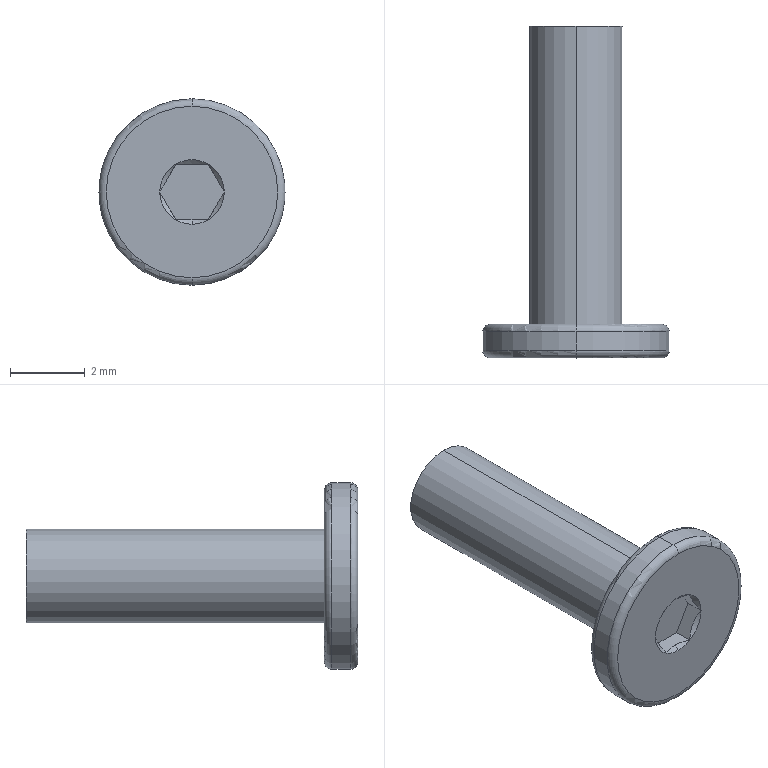Part | NX | features BREP 1 | 1 solid | 25 faces | box 5 x 8.9 x 5 mm | volume 55.675 mm3 | plane 10 | cone 7 | torus 4 | cylinder 4 | commonest cylinder face diameters 2.5 x2 5 x2
STEP:
#1=CARTESIAN_POINT('',(0.,0.7,-2.5));
#2=VERTEX_POINT('',#1);
#3=CARTESIAN_POINT('',(0.,0.7,2.5));
#4=VERTEX_POINT('',#3);
#5=CARTESIAN_POINT('',(0.,0.7,0.));
#6=DIRECTION('',(0.,-1.,0.));
#7=DIRECTION('',(0.,0.,1.));
#8=AXIS2_PLACEMENT_3D('',#5,#6,#7);
#9=CIRCLE('',#8,2.5);
#10=EDGE_CURVE('',#2,#4,#9,.T.);
#11=ORIENTED_EDGE('',*,*,#10,.F.);
#12=CARTESIAN_POINT('',(0.,0.9,-2.3));
#13=VERTEX_POINT('',#12);
#14=CARTESIAN_POINT('',(0.,0.7,-2.3));
#15=DIRECTION('',(1.,0.,0.));
#16=DIRECTION('',(0.,0.,-1.));
#17=AXIS2_PLACEMENT_3D('',#14,#15,#16);
#18=CIRCLE('',#17,0.2);
#19=EDGE_CURVE('',#2,#13,#18,.T.);
#20=ORIENTED_EDGE('',*,*,#19,.T.);
#21=CARTESIAN_POINT('',(0.,0.9,2.3));
#22=VERTEX_POINT('',#21);
#23=CARTESIAN_POINT('',(0.,0.9,0.));
#24=DIRECTION('',(0.,1.,0.));
#25=DIRECTION('',(0.,0.,1.));
#26=AXIS2_PLACEMENT_3D('',#23,#24,#25);
#27=CIRCLE('',#26,2.3);
#28=EDGE_CURVE('',#22,#13,#27,.T.);
#29=ORIENTED_EDGE('',*,*,#28,.F.);
#30=CARTESIAN_POINT('',(0.,0.7,2.3));
#31=DIRECTION('',(-1.,0.,0.));
#32=DIRECTION('',(0.,0.,1.));
#33=AXIS2_PLACEMENT_3D('',#30,#31,#32);
#34=CIRCLE('',#33,0.2);
#35=EDGE_CURVE('',#4,#22,#34,.T.);
#36=ORIENTED_EDGE('',*,*,#35,.F.);
#37=EDGE_LOOP('',(#11,#20,#29,#36));
#38=FACE_BOUND('',#37,.T.);
#39=CARTESIAN_POINT('',(0.,0.7,0.));
#40=DIRECTION('',(0.,1.,0.));
#41=DIRECTION('',(0.,0.,-1.));
#42=AXIS2_PLACEMENT_3D('',#39,#40,#41);
#43=TOROIDAL_SURFACE('',#42,2.3,0.2);
#44=ADVANCED_FACE('',(#38),#43,.T.);
#45=CARTESIAN_POINT('',(0.,0.,-2.3));
#46=VERTEX_POINT('',#45);
#47=CARTESIAN_POINT('',(0.,0.,2.3));
#48=VERTEX_POINT('',#47);
#49=CARTESIAN_POINT('',(0.,0.,0.));
#50=DIRECTION('',(0.,-1.,0.));
#51=DIRECTION('',(0.,0.,1.));
#52=AXIS2_PLACEMENT_3D('',#49,#50,#51);
#53=CIRCLE('',#52,2.3);
#54=EDGE_CURVE('',#46,#48,#53,.T.);
#55=ORIENTED_EDGE('',*,*,#54,.F.);
#56=CARTESIAN_POINT('',(0.,0.2,-2.5));
#57=VERTEX_POINT('',#56);
#58=CARTESIAN_POINT('',(0.,0.2,-2.3));
#59=DIRECTION('',(1.,0.,0.));
#60=DIRECTION('',(0.,0.,-1.));
#61=AXIS2_PLACEMENT_3D('',#58,#59,#60);
#62=CIRCLE('',#61,0.2);
#63=EDGE_CURVE('',#46,#57,#62,.T.);
#64=ORIENTED_EDGE('',*,*,#63,.T.);
#65=CARTESIAN_POINT('',(0.,0.2,2.5));
#66=VERTEX_POINT('',#65);
#67=CARTESIAN_POINT('',(0.,0.2,0.));
#68=DIRECTION('',(0.,1.,0.));
#69=DIRECTION('',(0.,0.,1.));
#70=AXIS2_PLACEMENT_3D('',#67,#68,#69);
#71=CIRCLE('',#70,2.5);
#72=EDGE_CURVE('',#66,#57,#71,.T.);
#73=ORIENTED_EDGE('',*,*,#72,.F.);
#74=CARTESIAN_POINT('',(0.,0.2,2.3));
#75=DIRECTION('',(-1.,0.,0.));
#76=DIRECTION('',(0.,0.,1.));
#77=AXIS2_PLACEMENT_3D('',#74,#75,#76);
#78=CIRCLE('',#77,0.2);
#79=EDGE_CURVE('',#48,#66,#78,.T.);
#80=ORIENTED_EDGE('',*,*,#79,.F.);
#81=EDGE_LOOP('',(#55,#64,#73,#80));
#82=FACE_BOUND('',#81,.T.);
#83=CARTESIAN_POINT('',(0.,0.2,0.));
#84=DIRECTION('',(0.,1.,0.));
#85=DIRECTION('',(0.,0.,-1.));
#86=AXIS2_PLACEMENT_3D('',#83,#84,#85);
#87=TOROIDAL_SURFACE('',#86,2.3,0.2);
#88=ADVANCED_FACE('',(#82),#87,.T.);
#89=CARTESIAN_POINT('',(0.,0.116,-0.75));
#90=VERTEX_POINT('',#89);
#91=CARTESIAN_POINT('',(0.433,0.,-0.75));
#92=VERTEX_POINT('',#91);
#93=CARTESIAN_POINT('',(0.,0.116,-0.75));
#94=CARTESIAN_POINT('',(0.1521,0.116,-0.75));
#95=CARTESIAN_POINT('',(0.2975,0.06775,-0.75));
#96=CARTESIAN_POINT('',(0.433,0.,-0.75));
#97=B_SPLINE_CURVE_WITH_KNOTS('',3,(#93,#94,#95,#96),.UNSPECIFIED.,.F.,.F.,(4,4),(0.,0.0004495),.UNSPECIFIED.);
#98=EDGE_CURVE('',#90,#92,#97,.T.);
#99=ORIENTED_EDGE('',*,*,#98,.F.);
#100=CARTESIAN_POINT('',(0.,0.,-0.866));
#101=VERTEX_POINT('',#100);
#102=CARTESIAN_POINT('',(0.,0.,-0.866));
#103=DIRECTION('',(0.,-0.7071,-0.7071));
#104=VECTOR('',#103,1000.);
#105=LINE('',#102,#104);
#106=EDGE_CURVE('',#90,#101,#105,.T.);
#107=ORIENTED_EDGE('',*,*,#106,.T.);
#108=CARTESIAN_POINT('',(0.,0.,0.));
#109=DIRECTION('',(0.,-1.,0.));
#110=DIRECTION('',(0.,0.,-1.));
#111=AXIS2_PLACEMENT_3D('',#108,#109,#110);
#112=CIRCLE('',#111,0.866);
#113=EDGE_CURVE('',#101,#92,#112,.T.);
#114=ORIENTED_EDGE('',*,*,#113,.T.);
#115=EDGE_LOOP('',(#99,#107,#114));
#116=FACE_BOUND('',#115,.T.);
#117=CARTESIAN_POINT('',(0.,0.,0.));
#118=DIRECTION('',(0.,-1.,0.));
#119=DIRECTION('',(0.,0.,1.));
#120=AXIS2_PLACEMENT_3D('',#117,#118,#119);
#121=CONICAL_SURFACE('',#120,0.866,0.7854);
#122=ADVANCED_FACE('',(#116),#121,.F.);
#123=CARTESIAN_POINT('',(0.,8.9,1.25));
#124=VERTEX_POINT('',#123);
#125=CARTESIAN_POINT('',(0.,8.9,-1.25));
#126=VERTEX_POINT('',#125);
#127=CARTESIAN_POINT('',(0.,8.9,0.));
#128=DIRECTION('',(0.,1.,0.));
#129=DIRECTION('',(0.,0.,1.));
#130=AXIS2_PLACEMENT_3D('',#127,#128,#129);
#131=CIRCLE('',#130,1.25);
#132=EDGE_CURVE('',#124,#126,#131,.T.);
#133=ORIENTED_EDGE('',*,*,#132,.F.);
#134=CARTESIAN_POINT('',(0.,0.9,1.25));
#135=VERTEX_POINT('',#134);
#136=CARTESIAN_POINT('',(0.,8.9,1.25));
#137=DIRECTION('',(0.,-1.,0.));
#138=VECTOR('',#137,1000.);
#139=LINE('',#136,#138);
#140=EDGE_CURVE('',#135,#124,#139,.F.);
#141=ORIENTED_EDGE('',*,*,#140,.F.);
#142=CARTESIAN_POINT('',(0.,0.9,-1.25));
#143=VERTEX_POINT('',#142);
#144=CARTESIAN_POINT('',(0.,0.9,0.));
#145=DIRECTION('',(0.,1.,0.));
#146=DIRECTION('',(0.,0.,1.));
#147=AXIS2_PLACEMENT_3D('',#144,#145,#146);
#148=CIRCLE('',#147,1.25);
#149=EDGE_CURVE('',#135,#143,#148,.T.);
#150=ORIENTED_EDGE('',*,*,#149,.T.);
#151=CARTESIAN_POINT('',(0.,8.9,-1.25));
#152=DIRECTION('',(0.,-1.,0.));
#153=VECTOR('',#152,1000.);
#154=LINE('',#151,#153);
#155=EDGE_CURVE('',#143,#126,#154,.F.);
#156=ORIENTED_EDGE('',*,*,#155,.T.);
#157=EDGE_LOOP('',(#133,#141,#150,#156));
#158=FACE_BOUND('',#157,.T.);
#159=CARTESIAN_POINT('',(0.,8.9,0.));
#160=DIRECTION('',(0.,-1.,0.));
#161=DIRECTION('',(0.,0.,1.));
#162=AXIS2_PLACEMENT_3D('',#159,#160,#161);
#163=CYLINDRICAL_SURFACE('',#162,1.25);
#164=ADVANCED_FACE('',(#158),#163,.T.);
#165=ORIENTED_EDGE('',*,*,#10,.T.);
#166=CARTESIAN_POINT('',(0.,0.9,2.5));
#167=DIRECTION('',(0.,-1.,0.));
#168=VECTOR('',#167,1000.);
#169=LINE('',#166,#168);
#170=EDGE_CURVE('',#66,#4,#169,.F.);
#171=ORIENTED_EDGE('',*,*,#170,.F.);
#172=ORIENTED_EDGE('',*,*,#72,.T.);
#173=CARTESIAN_POINT('',(0.,0.9,-2.5));
#174=DIRECTION('',(0.,-1.,0.));
#175=VECTOR('',#174,1000.);
#176=LINE('',#173,#175);
#177=EDGE_CURVE('',#57,#2,#176,.F.);
#178=ORIENTED_EDGE('',*,*,#177,.T.);
#179=EDGE_LOOP('',(#165,#171,#172,#178));
#180=FACE_BOUND('',#179,.T.);
#181=CARTESIAN_POINT('',(0.,0.9,0.));
#182=DIRECTION('',(0.,-1.,0.));
#183=DIRECTION('',(0.,0.,1.));
#184=AXIS2_PLACEMENT_3D('',#181,#182,#183);
#185=CYLINDRICAL_SURFACE('',#184,2.5);
#186=ADVANCED_FACE('',(#180),#185,.T.);
#187=ORIENTED_EDGE('',*,*,#170,.T.);
#188=CARTESIAN_POINT('',(0.,0.7,0.));
#189=DIRECTION('',(0.,-1.,0.));
#190=DIRECTION('',(0.,0.,1.));
#191=AXIS2_PLACEMENT_3D('',#188,#189,#190);
#192=CIRCLE('',#191,2.5);
#193=EDGE_CURVE('',#4,#2,#192,.T.);
#194=ORIENTED_EDGE('',*,*,#193,.T.);
#195=ORIENTED_EDGE('',*,*,#177,.F.);
#196=CARTESIAN_POINT('',(0.,0.2,0.));
#197=DIRECTION('',(0.,1.,0.));
#198=DIRECTION('',(0.,0.,1.));
#199=AXIS2_PLACEMENT_3D('',#196,#197,#198);
#200=CIRCLE('',#199,2.5);
#201=EDGE_CURVE('',#57,#66,#200,.T.);
#202=ORIENTED_EDGE('',*,*,#201,.T.);
#203=EDGE_LOOP('',(#187,#194,#195,#202));
#204=FACE_BOUND('',#203,.T.);
#205=CARTESIAN_POINT('',(0.,0.9,0.));
#206=DIRECTION('',(0.,-1.,0.));
#207=DIRECTION('',(0.,0.,1.));
#208=AXIS2_PLACEMENT_3D('',#205,#206,#207);
#209=CYLINDRICAL_SURFACE('',#208,2.5);
#210=ADVANCED_FACE('',(#204),#209,.T.);
#211=ORIENTED_EDGE('',*,*,#28,.T.);
#212=CARTESIAN_POINT('',(0.,0.9,0.));
#213=DIRECTION('',(0.,1.,0.));
#214=DIRECTION('',(0.,0.,1.));
#215=AXIS2_PLACEMENT_3D('',#212,#213,#214);
#216=CIRCLE('',#215,2.3);
#217=EDGE_CURVE('',#13,#22,#216,.T.);
#218=ORIENTED_EDGE('',*,*,#217,.T.);
#219=EDGE_LOOP('',(#211,#218));
#220=FACE_BOUND('',#219,.T.);
#221=CARTESIAN_POINT('',(0.,0.9,0.));
#222=DIRECTION('',(0.,1.,0.));
#223=DIRECTION('',(0.,0.,1.));
#224=AXIS2_PLACEMENT_3D('',#221,#222,#223);
#225=CIRCLE('',#224,1.25);
#226=EDGE_CURVE('',#143,#135,#225,.T.);
#227=ORIENTED_EDGE('',*,*,#226,.F.);
#228=ORIENTED_EDGE('',*,*,#149,.F.);
#229=EDGE_LOOP('',(#227,#228));
#230=FACE_BOUND('',#229,.T.);
#231=CARTESIAN_POINT('',(0.,0.9,0.));
#232=DIRECTION('',(0.,1.,0.));
#233=DIRECTION('',(-1.,0.,0.));
#234=AXIS2_PLACEMENT_3D('',#231,#232,#233);
#235=PLANE('',#234);
#236=ADVANCED_FACE('',(#220,#230),#235,.T.);
#237=CARTESIAN_POINT('',(0.,0.,0.));
#238=DIRECTION('',(0.,-1.,0.));
#239=DIRECTION('',(0.,0.,1.));
#240=AXIS2_PLACEMENT_3D('',#237,#238,#239);
#241=CIRCLE('',#240,2.3);
#242=EDGE_CURVE('',#48,#46,#241,.T.);
#243=ORIENTED_EDGE('',*,*,#242,.T.);
#244=ORIENTED_EDGE('',*,*,#54,.T.);
#245=EDGE_LOOP('',(#243,#244));
#246=FACE_BOUND('',#245,.T.);
#247=CARTESIAN_POINT('',(0.433,0.,0.75));
#248=VERTEX_POINT('',#247);
#249=CARTESIAN_POINT('',(-0.433,0.,0.75));
#250=VERTEX_POINT('',#249);
#251=CARTESIAN_POINT('',(0.,0.,0.));
#252=DIRECTION('',(0.,-1.,0.));
#253=DIRECTION('',(0.,0.,-1.));
#254=AXIS2_PLACEMENT_3D('',#251,#252,#253);
#255=CIRCLE('',#254,0.866);
#256=EDGE_CURVE('',#248,#250,#255,.T.);
#257=ORIENTED_EDGE('',*,*,#256,.F.);
#258=CARTESIAN_POINT('',(0.866,0.,0.));
#259=VERTEX_POINT('',#258);
#260=CARTESIAN_POINT('',(0.,0.,0.));
#261=DIRECTION('',(0.,-1.,0.));
#262=DIRECTION('',(0.,0.,-1.));
#263=AXIS2_PLACEMENT_3D('',#260,#261,#262);
#264=CIRCLE('',#263,0.866);
#265=EDGE_CURVE('',#259,#248,#264,.T.);
#266=ORIENTED_EDGE('',*,*,#265,.F.);
#267=CARTESIAN_POINT('',(0.,0.,0.));
#268=DIRECTION('',(0.,-1.,0.));
#269=DIRECTION('',(0.,0.,-1.));
#270=AXIS2_PLACEMENT_3D('',#267,#268,#269);
#271=CIRCLE('',#270,0.866);
#272=EDGE_CURVE('',#92,#259,#271,.T.);
#273=ORIENTED_EDGE('',*,*,#272,.F.);
#274=ORIENTED_EDGE('',*,*,#113,.F.);
#275=CARTESIAN_POINT('',(-0.433,0.,-0.75));
#276=VERTEX_POINT('',#275);
#277=CARTESIAN_POINT('',(0.,0.,0.));
#278=DIRECTION('',(0.,-1.,0.));
#279=DIRECTION('',(0.,0.,-1.));
#280=AXIS2_PLACEMENT_3D('',#277,#278,#279);
#281=CIRCLE('',#280,0.866);
#282=EDGE_CURVE('',#276,#101,#281,.T.);
#283=ORIENTED_EDGE('',*,*,#282,.F.);
#284=CARTESIAN_POINT('',(-0.866,0.,0.));
#285=VERTEX_POINT('',#284);
#286=CARTESIAN_POINT('',(0.,0.,0.));
#287=DIRECTION('',(0.,-1.,0.));
#288=DIRECTION('',(0.,0.,-1.));
#289=AXIS2_PLACEMENT_3D('',#286,#287,#288);
#290=CIRCLE('',#289,0.866);
#291=EDGE_CURVE('',#285,#276,#290,.T.);
#292=ORIENTED_EDGE('',*,*,#291,.F.);
#293=CARTESIAN_POINT('',(0.,0.,0.));
#294=DIRECTION('',(0.,-1.,0.));
#295=DIRECTION('',(0.,0.,-1.));
#296=AXIS2_PLACEMENT_3D('',#293,#294,#295);
#297=CIRCLE('',#296,0.866);
#298=EDGE_CURVE('',#250,#285,#297,.T.);
#299=ORIENTED_EDGE('',*,*,#298,.F.);
#300=EDGE_LOOP('',(#257,#266,#273,#274,#283,#292,#299));
#301=FACE_BOUND('',#300,.T.);
#302=CARTESIAN_POINT('',(0.,0.,0.));
#303=DIRECTION('',(0.,1.,0.));
#304=DIRECTION('',(-1.,0.,0.));
#305=AXIS2_PLACEMENT_3D('',#302,#303,#304);
#306=PLANE('',#305);
#307=ADVANCED_FACE('',(#246,#301),#306,.F.);
#308=ORIENTED_EDGE('',*,*,#140,.T.);
#309=CARTESIAN_POINT('',(0.,8.9,0.));
#310=DIRECTION('',(0.,1.,0.));
#311=DIRECTION('',(0.,0.,1.));
#312=AXIS2_PLACEMENT_3D('',#309,#310,#311);
#313=CIRCLE('',#312,1.25);
#314=EDGE_CURVE('',#126,#124,#313,.T.);
#315=ORIENTED_EDGE('',*,*,#314,.F.);
#316=ORIENTED_EDGE('',*,*,#155,.F.);
#317=ORIENTED_EDGE('',*,*,#226,.T.);
#318=EDGE_LOOP('',(#308,#315,#316,#317));
#319=FACE_BOUND('',#318,.T.);
#320=CARTESIAN_POINT('',(0.,8.9,0.));
#321=DIRECTION('',(0.,-1.,0.));
#322=DIRECTION('',(0.,0.,1.));
#323=AXIS2_PLACEMENT_3D('',#320,#321,#322);
#324=CYLINDRICAL_SURFACE('',#323,1.25);
#325=ADVANCED_FACE('',(#319),#324,.T.);
#326=ORIENTED_EDGE('',*,*,#314,.T.);
#327=ORIENTED_EDGE('',*,*,#132,.T.);
#328=EDGE_LOOP('',(#326,#327));
#329=FACE_BOUND('',#328,.T.);
#330=CARTESIAN_POINT('',(0.,8.9,0.));
#331=DIRECTION('',(0.,1.,0.));
#332=DIRECTION('',(-1.,0.,0.));
#333=AXIS2_PLACEMENT_3D('',#330,#331,#332);
#334=PLANE('',#333);
#335=ADVANCED_FACE('',(#329),#334,.T.);
#336=ORIENTED_EDGE('',*,*,#265,.T.);
#337=CARTESIAN_POINT('',(0.866,0.,0.));
#338=CARTESIAN_POINT('',(0.7307,0.1353,0.2344));
#339=CARTESIAN_POINT('',(0.5691,0.1361,0.5142));
#340=CARTESIAN_POINT('',(0.433,0.,0.75));
#341=B_SPLINE_CURVE_WITH_KNOTS('',3,(#337,#338,#339,#340),.UNSPECIFIED.,.F.,.F.,(4,4),(0.,0.0008946),.UNSPECIFIED.);
#342=EDGE_CURVE('',#259,#248,#341,.T.);
#343=ORIENTED_EDGE('',*,*,#342,.F.);
#344=EDGE_LOOP('',(#336,#343));
#345=FACE_BOUND('',#344,.T.);
#346=CARTESIAN_POINT('',(0.,0.,0.));
#347=DIRECTION('',(0.,-1.,0.));
#348=DIRECTION('',(0.,0.,1.));
#349=AXIS2_PLACEMENT_3D('',#346,#347,#348);
#350=CONICAL_SURFACE('',#349,0.866,0.7854);
#351=ADVANCED_FACE('',(#345),#350,.F.);
#352=ORIENTED_EDGE('',*,*,#256,.T.);
#353=CARTESIAN_POINT('',(0.433,0.,0.75));
#354=CARTESIAN_POINT('',(0.1624,0.1353,0.75));
#355=CARTESIAN_POINT('',(-0.1608,0.1361,0.75));
#356=CARTESIAN_POINT('',(-0.433,0.,0.75));
#357=B_SPLINE_CURVE_WITH_KNOTS('',3,(#353,#354,#355,#356),.UNSPECIFIED.,.F.,.F.,(4,4),(0.,0.0008946),.UNSPECIFIED.);
#358=EDGE_CURVE('',#248,#250,#357,.T.);
#359=ORIENTED_EDGE('',*,*,#358,.F.);
#360=EDGE_LOOP('',(#352,#359));
#361=FACE_BOUND('',#360,.T.);
#362=CARTESIAN_POINT('',(0.,0.,0.));
#363=DIRECTION('',(0.,-1.,0.));
#364=DIRECTION('',(0.,0.,1.));
#365=AXIS2_PLACEMENT_3D('',#362,#363,#364);
#366=CONICAL_SURFACE('',#365,0.866,0.7854);
#367=ADVANCED_FACE('',(#361),#366,.F.);
#368=ORIENTED_EDGE('',*,*,#298,.T.);
#369=CARTESIAN_POINT('',(-0.433,0.,0.75));
#370=CARTESIAN_POINT('',(-0.5683,0.1353,0.5156));
#371=CARTESIAN_POINT('',(-0.7299,0.1361,0.2358));
#372=CARTESIAN_POINT('',(-0.866,0.,0.));
#373=B_SPLINE_CURVE_WITH_KNOTS('',3,(#369,#370,#371,#372),.UNSPECIFIED.,.F.,.F.,(4,4),(0.,0.0008946),.UNSPECIFIED.);
#374=EDGE_CURVE('',#250,#285,#373,.T.);
#375=ORIENTED_EDGE('',*,*,#374,.F.);
#376=EDGE_LOOP('',(#368,#375));
#377=FACE_BOUND('',#376,.T.);
#378=CARTESIAN_POINT('',(0.,0.,0.));
#379=DIRECTION('',(0.,-1.,0.));
#380=DIRECTION('',(0.,0.,1.));
#381=AXIS2_PLACEMENT_3D('',#378,#379,#380);
#382=CONICAL_SURFACE('',#381,0.866,0.7854);
#383=ADVANCED_FACE('',(#377),#382,.F.);
#384=ORIENTED_EDGE('',*,*,#291,.T.);
#385=CARTESIAN_POINT('',(-0.866,0.,0.));
#386=CARTESIAN_POINT('',(-0.7307,0.1353,-0.2344));
#387=CARTESIAN_POINT('',(-0.5691,0.1361,-0.5142));
#388=CARTESIAN_POINT('',(-0.433,0.,-0.75));
#389=B_SPLINE_CURVE_WITH_KNOTS('',3,(#385,#386,#387,#388),.UNSPECIFIED.,.F.,.F.,(4,4),(0.,0.0008946),.UNSPECIFIED.);
#390=EDGE_CURVE('',#285,#276,#389,.T.);
#391=ORIENTED_EDGE('',*,*,#390,.F.);
#392=EDGE_LOOP('',(#384,#391));
#393=FACE_BOUND('',#392,.T.);
#394=CARTESIAN_POINT('',(0.,0.,0.));
#395=DIRECTION('',(0.,-1.,0.));
#396=DIRECTION('',(0.,0.,1.));
#397=AXIS2_PLACEMENT_3D('',#394,#395,#396);
#398=CONICAL_SURFACE('',#397,0.866,0.7854);
#399=ADVANCED_FACE('',(#393),#398,.F.);
#400=ORIENTED_EDGE('',*,*,#106,.F.);
#401=CARTESIAN_POINT('',(-0.433,0.,-0.75));
#402=CARTESIAN_POINT('',(-0.2973,0.06786,-0.75));
#403=CARTESIAN_POINT('',(-0.1532,0.116,-0.75));
#404=CARTESIAN_POINT('',(0.,0.116,-0.75));
#405=B_SPLINE_CURVE_WITH_KNOTS('',3,(#401,#402,#403,#404),.UNSPECIFIED.,.F.,.F.,(4,4),(0.,0.0004486),.UNSPECIFIED.);
#406=EDGE_CURVE('',#276,#90,#405,.T.);
#407=ORIENTED_EDGE('',*,*,#406,.F.);
#408=ORIENTED_EDGE('',*,*,#282,.T.);
#409=EDGE_LOOP('',(#400,#407,#408));
#410=FACE_BOUND('',#409,.T.);
#411=CARTESIAN_POINT('',(0.,0.,0.));
#412=DIRECTION('',(0.,-1.,0.));
#413=DIRECTION('',(0.,0.,1.));
#414=AXIS2_PLACEMENT_3D('',#411,#412,#413);
#415=CONICAL_SURFACE('',#414,0.866,0.7854);
#416=ADVANCED_FACE('',(#410),#415,.F.);
#417=ORIENTED_EDGE('',*,*,#272,.T.);
#418=CARTESIAN_POINT('',(0.433,0.,-0.75));
#419=CARTESIAN_POINT('',(0.5683,0.1353,-0.5156));
#420=CARTESIAN_POINT('',(0.7299,0.1361,-0.2358));
#421=CARTESIAN_POINT('',(0.866,0.,0.));
#422=B_SPLINE_CURVE_WITH_KNOTS('',3,(#418,#419,#420,#421),.UNSPECIFIED.,.F.,.F.,(4,4),(0.,0.0008946),.UNSPECIFIED.);
#423=EDGE_CURVE('',#92,#259,#422,.T.);
#424=ORIENTED_EDGE('',*,*,#423,.F.);
#425=EDGE_LOOP('',(#417,#424));
#426=FACE_BOUND('',#425,.T.);
#427=CARTESIAN_POINT('',(0.,0.,0.));
#428=DIRECTION('',(0.,-1.,0.));
#429=DIRECTION('',(0.,0.,1.));
#430=AXIS2_PLACEMENT_3D('',#427,#428,#429);
#431=CONICAL_SURFACE('',#430,0.866,0.7854);
#432=ADVANCED_FACE('',(#426),#431,.F.);
#433=CARTESIAN_POINT('',(0.433,0.5,-0.75));
#434=VERTEX_POINT('',#433);
#435=CARTESIAN_POINT('',(0.866,0.5,0.));
#436=VERTEX_POINT('',#435);
#437=CARTESIAN_POINT('',(0.433,0.5,-0.75));
#438=DIRECTION('',(0.5,0.,0.866));
#439=VECTOR('',#438,1000.);
#440=LINE('',#437,#439);
#441=EDGE_CURVE('',#434,#436,#440,.T.);
#442=ORIENTED_EDGE('',*,*,#441,.T.);
#443=CARTESIAN_POINT('',(0.433,0.5,0.75));
#444=VERTEX_POINT('',#443);
#445=CARTESIAN_POINT('',(0.866,0.5,0.));
#446=DIRECTION('',(-0.5,0.,0.866));
#447=VECTOR('',#446,1000.);
#448=LINE('',#445,#447);
#449=EDGE_CURVE('',#436,#444,#448,.T.);
#450=ORIENTED_EDGE('',*,*,#449,.T.);
#451=CARTESIAN_POINT('',(-0.433,0.5,0.75));
#452=VERTEX_POINT('',#451);
#453=CARTESIAN_POINT('',(0.433,0.5,0.75));
#454=DIRECTION('',(-1.,0.,0.));
#455=VECTOR('',#454,1000.);
#456=LINE('',#453,#455);
#457=EDGE_CURVE('',#444,#452,#456,.T.);
#458=ORIENTED_EDGE('',*,*,#457,.T.);
#459=CARTESIAN_POINT('',(-0.866,0.5,0.));
#460=VERTEX_POINT('',#459);
#461=CARTESIAN_POINT('',(-0.433,0.5,0.75));
#462=DIRECTION('',(-0.5,0.,-0.866));
#463=VECTOR('',#462,1000.);
#464=LINE('',#461,#463);
#465=EDGE_CURVE('',#452,#460,#464,.T.);
#466=ORIENTED_EDGE('',*,*,#465,.T.);
#467=CARTESIAN_POINT('',(-0.433,0.5,-0.75));
#468=VERTEX_POINT('',#467);
#469=CARTESIAN_POINT('',(-0.866,0.5,0.));
#470=DIRECTION('',(0.5,0.,-0.866));
#471=VECTOR('',#470,1000.);
#472=LINE('',#469,#471);
#473=EDGE_CURVE('',#460,#468,#472,.T.);
#474=ORIENTED_EDGE('',*,*,#473,.T.);
#475=CARTESIAN_POINT('',(-0.433,0.5,-0.75));
#476=DIRECTION('',(1.,0.,0.));
#477=VECTOR('',#476,1000.);
#478=LINE('',#475,#477);
#479=EDGE_CURVE('',#468,#434,#478,.T.);
#480=ORIENTED_EDGE('',*,*,#479,.T.);
#481=EDGE_LOOP('',(#442,#450,#458,#466,#474,#480));
#482=FACE_BOUND('',#481,.T.);
#483=CARTESIAN_POINT('',(0.,0.5,0.));
#484=DIRECTION('',(0.,-1.,0.));
#485=DIRECTION('',(0.,0.,1.));
#486=AXIS2_PLACEMENT_3D('',#483,#484,#485);
#487=PLANE('',#486);
#488=ADVANCED_FACE('',(#482),#487,.T.);
#489=CARTESIAN_POINT('',(0.866,0.5,0.));
#490=DIRECTION('',(0.,-1.,0.));
#491=VECTOR('',#490,1000.);
#492=LINE('',#489,#491);
#493=EDGE_CURVE('',#436,#259,#492,.T.);
#494=ORIENTED_EDGE('',*,*,#493,.T.);
#495=ORIENTED_EDGE('',*,*,#342,.T.);
#496=CARTESIAN_POINT('',(0.433,0.5,0.75));
#497=DIRECTION('',(0.,-1.,0.));
#498=VECTOR('',#497,1000.);
#499=LINE('',#496,#498);
#500=EDGE_CURVE('',#444,#248,#499,.T.);
#501=ORIENTED_EDGE('',*,*,#500,.F.);
#502=ORIENTED_EDGE('',*,*,#449,.F.);
#503=EDGE_LOOP('',(#494,#495,#501,#502));
#504=FACE_BOUND('',#503,.T.);
#505=CARTESIAN_POINT('',(0.866,0.5,0.));
#506=DIRECTION('',(0.866,0.,0.5));
#507=DIRECTION('',(0.,1.,0.));
#508=AXIS2_PLACEMENT_3D('',#505,#506,#507);
#509=PLANE('',#508);
#510=ADVANCED_FACE('',(#504),#509,.F.);
#511=ORIENTED_EDGE('',*,*,#500,.T.);
#512=ORIENTED_EDGE('',*,*,#358,.T.);
#513=CARTESIAN_POINT('',(-0.433,0.5,0.75));
#514=DIRECTION('',(0.,-1.,0.));
#515=VECTOR('',#514,1000.);
#516=LINE('',#513,#515);
#517=EDGE_CURVE('',#452,#250,#516,.T.);
#518=ORIENTED_EDGE('',*,*,#517,.F.);
#519=ORIENTED_EDGE('',*,*,#457,.F.);
#520=EDGE_LOOP('',(#511,#512,#518,#519));
#521=FACE_BOUND('',#520,.T.);
#522=CARTESIAN_POINT('',(0.433,0.5,0.75));
#523=DIRECTION('',(0.,0.,1.));
#524=DIRECTION('',(-1.,0.,0.));
#525=AXIS2_PLACEMENT_3D('',#522,#523,#524);
#526=PLANE('',#525);
#527=ADVANCED_FACE('',(#521),#526,.F.);
#528=ORIENTED_EDGE('',*,*,#517,.T.);
#529=ORIENTED_EDGE('',*,*,#374,.T.);
#530=CARTESIAN_POINT('',(-0.866,0.5,0.));
#531=DIRECTION('',(0.,-1.,0.));
#532=VECTOR('',#531,1000.);
#533=LINE('',#530,#532);
#534=EDGE_CURVE('',#460,#285,#533,.T.);
#535=ORIENTED_EDGE('',*,*,#534,.F.);
#536=ORIENTED_EDGE('',*,*,#465,.F.);
#537=EDGE_LOOP('',(#528,#529,#535,#536));
#538=FACE_BOUND('',#537,.T.);
#539=CARTESIAN_POINT('',(-0.433,0.5,0.75));
#540=DIRECTION('',(-0.866,0.,0.5));
#541=DIRECTION('',(0.,-1.,0.));
#542=AXIS2_PLACEMENT_3D('',#539,#540,#541);
#543=PLANE('',#542);
#544=ADVANCED_FACE('',(#538),#543,.F.);
#545=ORIENTED_EDGE('',*,*,#534,.T.);
#546=ORIENTED_EDGE('',*,*,#390,.T.);
#547=CARTESIAN_POINT('',(-0.433,0.5,-0.75));
#548=DIRECTION('',(0.,-1.,0.));
#549=VECTOR('',#548,1000.);
#550=LINE('',#547,#549);
#551=EDGE_CURVE('',#468,#276,#550,.T.);
#552=ORIENTED_EDGE('',*,*,#551,.F.);
#553=ORIENTED_EDGE('',*,*,#473,.F.);
#554=EDGE_LOOP('',(#545,#546,#552,#553));
#555=FACE_BOUND('',#554,.T.);
#556=CARTESIAN_POINT('',(-0.866,0.5,0.));
#557=DIRECTION('',(-0.866,0.,-0.5));
#558=DIRECTION('',(0.5,0.,-0.866));
#559=AXIS2_PLACEMENT_3D('',#556,#557,#558);
#560=PLANE('',#559);
#561=ADVANCED_FACE('',(#555),#560,.F.);
#562=ORIENTED_EDGE('',*,*,#551,.T.);
#563=ORIENTED_EDGE('',*,*,#406,.T.);
#564=ORIENTED_EDGE('',*,*,#98,.T.);
#565=CARTESIAN_POINT('',(0.433,0.5,-0.75));
#566=DIRECTION('',(0.,-1.,0.));
#567=VECTOR('',#566,1000.);
#568=LINE('',#565,#567);
#569=EDGE_CURVE('',#434,#92,#568,.T.);
#570=ORIENTED_EDGE('',*,*,#569,.F.);
#571=ORIENTED_EDGE('',*,*,#479,.F.);
#572=EDGE_LOOP('',(#562,#563,#564,#570,#571));
#573=FACE_BOUND('',#572,.T.);
#574=CARTESIAN_POINT('',(-0.433,0.5,-0.75));
#575=DIRECTION('',(0.,0.,-1.));
#576=DIRECTION('',(0.,1.,0.));
#577=AXIS2_PLACEMENT_3D('',#574,#575,#576);
#578=PLANE('',#577);
#579=ADVANCED_FACE('',(#573),#578,.F.);
#580=ORIENTED_EDGE('',*,*,#569,.T.);
#581=ORIENTED_EDGE('',*,*,#423,.T.);
#582=ORIENTED_EDGE('',*,*,#493,.F.);
#583=ORIENTED_EDGE('',*,*,#441,.F.);
#584=EDGE_LOOP('',(#580,#581,#582,#583));
#585=FACE_BOUND('',#584,.T.);
#586=CARTESIAN_POINT('',(0.433,0.5,-0.75));
#587=DIRECTION('',(0.866,0.,-0.5));
#588=DIRECTION('',(0.,1.,0.));
#589=AXIS2_PLACEMENT_3D('',#586,#587,#588);
#590=PLANE('',#589);
#591=ADVANCED_FACE('',(#585),#590,.F.);
#592=ORIENTED_EDGE('',*,*,#63,.F.);
#593=ORIENTED_EDGE('',*,*,#242,.F.);
#594=ORIENTED_EDGE('',*,*,#79,.T.);
#595=ORIENTED_EDGE('',*,*,#201,.F.);
#596=EDGE_LOOP('',(#592,#593,#594,#595));
#597=FACE_BOUND('',#596,.T.);
#598=CARTESIAN_POINT('',(0.,0.2,0.));
#599=DIRECTION('',(0.,1.,0.));
#600=DIRECTION('',(0.,0.,-1.));
#601=AXIS2_PLACEMENT_3D('',#598,#599,#600);
#602=TOROIDAL_SURFACE('',#601,2.3,0.2);
#603=ADVANCED_FACE('',(#597),#602,.T.);
#604=ORIENTED_EDGE('',*,*,#19,.F.);
#605=ORIENTED_EDGE('',*,*,#193,.F.);
#606=ORIENTED_EDGE('',*,*,#35,.T.);
#607=ORIENTED_EDGE('',*,*,#217,.F.);
#608=EDGE_LOOP('',(#604,#605,#606,#607));
#609=FACE_BOUND('',#608,.T.);
#610=CARTESIAN_POINT('',(0.,0.7,0.));
#611=DIRECTION('',(0.,1.,0.));
#612=DIRECTION('',(0.,0.,-1.));
#613=AXIS2_PLACEMENT_3D('',#610,#611,#612);
#614=TOROIDAL_SURFACE('',#613,2.3,0.2);
#615=ADVANCED_FACE('',(#609),#614,.T.);
#616=CLOSED_SHELL('',(#44,#88,#122,#164,#186,#210,#236,#307,#325,#335,#351,#367,#383,#399,#416,#432,#488,#510,#527,#544,#561,#579,#591,#603,#615));
#617=MANIFOLD_SOLID_BREP('',#616);
#618=(LENGTH_UNIT()NAMED_UNIT(*)SI_UNIT(.MILLI.,.METRE.));
#619=UNCERTAINTY_MEASURE_WITH_UNIT(LENGTH_MEASURE(0.0508),#618,'','');
#620=(NAMED_UNIT(*)PLANE_ANGLE_UNIT()SI_UNIT($,.RADIAN.));
#621=(NAMED_UNIT(*)SI_UNIT($,.STERADIAN.)SOLID_ANGLE_UNIT());
#622=(GEOMETRIC_REPRESENTATION_CONTEXT(3)GLOBAL_UNCERTAINTY_ASSIGNED_CONTEXT((#619))GLOBAL_UNIT_ASSIGNED_CONTEXT((#618,#620,#621))REPRESENTATION_CONTEXT('',''));
#623=ADVANCED_BREP_SHAPE_REPRESENTATION('',(#617),#622);